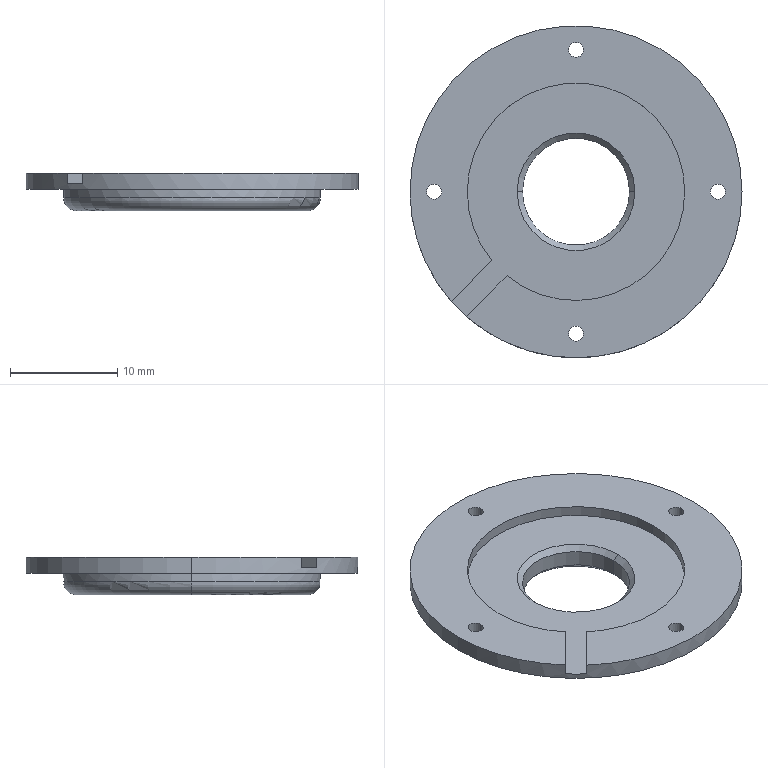Part | SolidWorks | features ICE 5, Chamfer 1, Extrusion 1, Fillet 1 | 1 solid | 41 faces | box 31 x 31 x 3.5 mm | volume 1459 mm3 | cylinder 25 | plane 10 | cone 4 | torus 2 | commonest cylinder face diameters 1.4 x8 2.5 x8 20.3 x3 10 x2 24 x2 31 x2
STEP:
#1=CARTESIAN_POINT('',(-5.,0.,2.));
#2=VERTEX_POINT('',#1);
#3=CARTESIAN_POINT('',(5.,0.,2.));
#4=VERTEX_POINT('',#3);
#5=CARTESIAN_POINT('',(0.,0.,2.));
#6=DIRECTION('',(0.,0.,1.));
#7=DIRECTION('',(1.,0.,0.));
#8=AXIS2_PLACEMENT_3D('',#5,#6,#7);
#9=CIRCLE('',#8,5.);
#10=EDGE_CURVE('',#2,#4,#9,.T.);
#11=ORIENTED_EDGE('',*,*,#10,.F.);
#12=CARTESIAN_POINT('',(-5.5,0.,2.5));
#13=VERTEX_POINT('',#12);
#14=CARTESIAN_POINT('',(-5.,0.,2.));
#15=DIRECTION('',(-0.7071,0.,0.7071));
#16=VECTOR('',#15,1000.);
#17=LINE('',#14,#16);
#18=EDGE_CURVE('',#2,#13,#17,.T.);
#19=ORIENTED_EDGE('',*,*,#18,.T.);
#20=CARTESIAN_POINT('',(5.5,0.,2.5));
#21=VERTEX_POINT('',#20);
#22=CARTESIAN_POINT('',(0.,0.,2.5));
#23=DIRECTION('',(0.,0.,-1.));
#24=DIRECTION('',(1.,0.,0.));
#25=AXIS2_PLACEMENT_3D('',#22,#23,#24);
#26=CIRCLE('',#25,5.5);
#27=EDGE_CURVE('',#21,#13,#26,.T.);
#28=ORIENTED_EDGE('',*,*,#27,.F.);
#29=CARTESIAN_POINT('',(5.,0.,2.));
#30=DIRECTION('',(0.7071,0.,0.7071));
#31=VECTOR('',#30,1000.);
#32=LINE('',#29,#31);
#33=EDGE_CURVE('',#4,#21,#32,.T.);
#34=ORIENTED_EDGE('',*,*,#33,.F.);
#35=EDGE_LOOP('',(#11,#19,#28,#34));
#36=FACE_OUTER_BOUND('',#35,.T.);
#37=CARTESIAN_POINT('',(0.,0.,2.));
#38=DIRECTION('',(0.,0.,1.));
#39=DIRECTION('',(1.,0.,0.));
#40=AXIS2_PLACEMENT_3D('',#37,#38,#39);
#41=CONICAL_SURFACE('',#40,5.,0.7854);
#42=ADVANCED_FACE('',(#36),#41,.F.);
#43=CARTESIAN_POINT('',(5.,0.,0.5));
#44=VERTEX_POINT('',#43);
#45=CARTESIAN_POINT('',(-5.,0.,0.5));
#46=VERTEX_POINT('',#45);
#47=CARTESIAN_POINT('',(0.,0.,0.5));
#48=DIRECTION('',(0.,0.,-1.));
#49=DIRECTION('',(1.,0.,0.));
#50=AXIS2_PLACEMENT_3D('',#47,#48,#49);
#51=CIRCLE('',#50,5.);
#52=EDGE_CURVE('',#44,#46,#51,.T.);
#53=ORIENTED_EDGE('',*,*,#52,.F.);
#54=CARTESIAN_POINT('',(5.5,0.,0.));
#55=VERTEX_POINT('',#54);
#56=CARTESIAN_POINT('',(5.,0.,0.5));
#57=DIRECTION('',(0.7071,0.,-0.7071));
#58=VECTOR('',#57,1000.);
#59=LINE('',#56,#58);
#60=EDGE_CURVE('',#44,#55,#59,.T.);
#61=ORIENTED_EDGE('',*,*,#60,.T.);
#62=CARTESIAN_POINT('',(-5.5,0.,0.));
#63=VERTEX_POINT('',#62);
#64=CARTESIAN_POINT('',(0.,0.,0.));
#65=DIRECTION('',(0.,0.,1.));
#66=DIRECTION('',(1.,0.,0.));
#67=AXIS2_PLACEMENT_3D('',#64,#65,#66);
#68=CIRCLE('',#67,5.5);
#69=EDGE_CURVE('',#63,#55,#68,.T.);
#70=ORIENTED_EDGE('',*,*,#69,.F.);
#71=CARTESIAN_POINT('',(-5.,0.,0.5));
#72=DIRECTION('',(-0.7071,0.,-0.7071));
#73=VECTOR('',#72,1000.);
#74=LINE('',#71,#73);
#75=EDGE_CURVE('',#46,#63,#74,.T.);
#76=ORIENTED_EDGE('',*,*,#75,.F.);
#77=EDGE_LOOP('',(#53,#61,#70,#76));
#78=FACE_OUTER_BOUND('',#77,.T.);
#79=CARTESIAN_POINT('',(0.,0.,0.5));
#80=DIRECTION('',(0.,0.,-1.));
#81=DIRECTION('',(-1.,0.,0.));
#82=AXIS2_PLACEMENT_3D('',#79,#80,#81);
#83=CONICAL_SURFACE('',#82,5.,0.7854);
#84=ADVANCED_FACE('',(#78),#83,.F.);
#85=ORIENTED_EDGE('',*,*,#10,.T.);
#86=CARTESIAN_POINT('',(5.,0.,3.5));
#87=DIRECTION('',(0.,0.,-1.));
#88=VECTOR('',#87,1000.);
#89=LINE('',#86,#88);
#90=EDGE_CURVE('',#4,#44,#89,.T.);
#91=ORIENTED_EDGE('',*,*,#90,.T.);
#92=ORIENTED_EDGE('',*,*,#52,.T.);
#93=CARTESIAN_POINT('',(-5.,0.,3.5));
#94=DIRECTION('',(0.,0.,-1.));
#95=VECTOR('',#94,1000.);
#96=LINE('',#93,#95);
#97=EDGE_CURVE('',#2,#46,#96,.T.);
#98=ORIENTED_EDGE('',*,*,#97,.F.);
#99=EDGE_LOOP('',(#85,#91,#92,#98));
#100=FACE_OUTER_BOUND('',#99,.T.);
#101=CARTESIAN_POINT('',(0.,0.,3.5));
#102=DIRECTION('',(0.,0.,-1.));
#103=DIRECTION('',(-1.,0.,0.));
#104=AXIS2_PLACEMENT_3D('',#101,#102,#103);
#105=CYLINDRICAL_SURFACE('',#104,5.);
#106=ADVANCED_FACE('',(#100),#105,.F.);
#107=CARTESIAN_POINT('',(1.25,13.25,2.5));
#108=VERTEX_POINT('',#107);
#109=CARTESIAN_POINT('',(-1.25,13.25,2.5));
#110=VERTEX_POINT('',#109);
#111=CARTESIAN_POINT('',(0.,13.25,2.5));
#112=DIRECTION('',(0.,0.,-1.));
#113=DIRECTION('',(-1.,0.,0.));
#114=AXIS2_PLACEMENT_3D('',#111,#112,#113);
#115=CIRCLE('',#114,1.25);
#116=EDGE_CURVE('',#108,#110,#115,.T.);
#117=ORIENTED_EDGE('',*,*,#116,.F.);
#118=CARTESIAN_POINT('',(1.25,13.25,2.));
#119=VERTEX_POINT('',#118);
#120=CARTESIAN_POINT('',(1.25,13.25,2.5));
#121=DIRECTION('',(0.,0.,-1.));
#122=VECTOR('',#121,1000.);
#123=LINE('',#120,#122);
#124=EDGE_CURVE('',#108,#119,#123,.T.);
#125=ORIENTED_EDGE('',*,*,#124,.T.);
#126=CARTESIAN_POINT('',(0.,12.,2.));
#127=VERTEX_POINT('',#126);
#128=CARTESIAN_POINT('',(0.,13.25,2.));
#129=DIRECTION('',(0.,0.,-1.));
#130=DIRECTION('',(-1.,0.,0.));
#131=AXIS2_PLACEMENT_3D('',#128,#129,#130);
#132=CIRCLE('',#131,1.25);
#133=EDGE_CURVE('',#119,#127,#132,.T.);
#134=ORIENTED_EDGE('',*,*,#133,.T.);
#135=CARTESIAN_POINT('',(-1.25,13.25,2.));
#136=VERTEX_POINT('',#135);
#137=CARTESIAN_POINT('',(0.,13.25,2.));
#138=DIRECTION('',(0.,0.,-1.));
#139=DIRECTION('',(-1.,0.,0.));
#140=AXIS2_PLACEMENT_3D('',#137,#138,#139);
#141=CIRCLE('',#140,1.25);
#142=EDGE_CURVE('',#127,#136,#141,.T.);
#143=ORIENTED_EDGE('',*,*,#142,.T.);
#144=CARTESIAN_POINT('',(-1.25,13.25,2.5));
#145=DIRECTION('',(0.,0.,-1.));
#146=VECTOR('',#145,1000.);
#147=LINE('',#144,#146);
#148=EDGE_CURVE('',#110,#136,#147,.T.);
#149=ORIENTED_EDGE('',*,*,#148,.F.);
#150=EDGE_LOOP('',(#117,#125,#134,#143,#149));
#151=FACE_OUTER_BOUND('',#150,.T.);
#152=CARTESIAN_POINT('',(0.,13.25,2.5));
#153=DIRECTION('',(0.,0.,-1.));
#154=DIRECTION('',(-1.,0.,0.));
#155=AXIS2_PLACEMENT_3D('',#152,#153,#154);
#156=CYLINDRICAL_SURFACE('',#155,1.25);
#157=ADVANCED_FACE('',(#151),#156,.F.);
#158=CARTESIAN_POINT('',(14.5,0.,2.5));
#159=VERTEX_POINT('',#158);
#160=CARTESIAN_POINT('',(12.,0.,2.5));
#161=VERTEX_POINT('',#160);
#162=CARTESIAN_POINT('',(13.25,0.,2.5));
#163=DIRECTION('',(0.,0.,-1.));
#164=DIRECTION('',(-1.,0.,0.));
#165=AXIS2_PLACEMENT_3D('',#162,#163,#164);
#166=CIRCLE('',#165,1.25);
#167=EDGE_CURVE('',#159,#161,#166,.T.);
#168=ORIENTED_EDGE('',*,*,#167,.F.);
#169=CARTESIAN_POINT('',(14.5,0.,2.));
#170=VERTEX_POINT('',#169);
#171=CARTESIAN_POINT('',(14.5,0.,2.5));
#172=DIRECTION('',(0.,0.,-1.));
#173=VECTOR('',#172,1000.);
#174=LINE('',#171,#173);
#175=EDGE_CURVE('',#159,#170,#174,.T.);
#176=ORIENTED_EDGE('',*,*,#175,.T.);
#177=CARTESIAN_POINT('',(12.,0.,2.));
#178=VERTEX_POINT('',#177);
#179=CARTESIAN_POINT('',(13.25,0.,2.));
#180=DIRECTION('',(0.,0.,-1.));
#181=DIRECTION('',(-1.,0.,0.));
#182=AXIS2_PLACEMENT_3D('',#179,#180,#181);
#183=CIRCLE('',#182,1.25);
#184=EDGE_CURVE('',#170,#178,#183,.T.);
#185=ORIENTED_EDGE('',*,*,#184,.T.);
#186=CARTESIAN_POINT('',(12.,0.,2.5));
#187=DIRECTION('',(0.,0.,-1.));
#188=VECTOR('',#187,1000.);
#189=LINE('',#186,#188);
#190=EDGE_CURVE('',#161,#178,#189,.T.);
#191=ORIENTED_EDGE('',*,*,#190,.F.);
#192=EDGE_LOOP('',(#168,#176,#185,#191));
#193=FACE_OUTER_BOUND('',#192,.T.);
#194=CARTESIAN_POINT('',(13.25,0.,2.5));
#195=DIRECTION('',(0.,0.,-1.));
#196=DIRECTION('',(-1.,0.,0.));
#197=AXIS2_PLACEMENT_3D('',#194,#195,#196);
#198=CYLINDRICAL_SURFACE('',#197,1.25);
#199=ADVANCED_FACE('',(#193),#198,.F.);
#200=CARTESIAN_POINT('',(1.25,-13.25,2.5));
#201=VERTEX_POINT('',#200);
#202=CARTESIAN_POINT('',(-1.25,-13.25,2.5));
#203=VERTEX_POINT('',#202);
#204=CARTESIAN_POINT('',(0.,-13.25,2.5));
#205=DIRECTION('',(0.,0.,-1.));
#206=DIRECTION('',(-1.,0.,0.));
#207=AXIS2_PLACEMENT_3D('',#204,#205,#206);
#208=CIRCLE('',#207,1.25);
#209=EDGE_CURVE('',#201,#203,#208,.T.);
#210=ORIENTED_EDGE('',*,*,#209,.F.);
#211=CARTESIAN_POINT('',(1.25,-13.25,2.));
#212=VERTEX_POINT('',#211);
#213=CARTESIAN_POINT('',(1.25,-13.25,2.5));
#214=DIRECTION('',(0.,0.,-1.));
#215=VECTOR('',#214,1000.);
#216=LINE('',#213,#215);
#217=EDGE_CURVE('',#201,#212,#216,.T.);
#218=ORIENTED_EDGE('',*,*,#217,.T.);
#219=CARTESIAN_POINT('',(-1.25,-13.25,2.));
#220=VERTEX_POINT('',#219);
#221=CARTESIAN_POINT('',(0.,-13.25,2.));
#222=DIRECTION('',(0.,0.,-1.));
#223=DIRECTION('',(-1.,0.,0.));
#224=AXIS2_PLACEMENT_3D('',#221,#222,#223);
#225=CIRCLE('',#224,1.25);
#226=EDGE_CURVE('',#212,#220,#225,.T.);
#227=ORIENTED_EDGE('',*,*,#226,.T.);
#228=CARTESIAN_POINT('',(-1.25,-13.25,2.5));
#229=DIRECTION('',(0.,0.,-1.));
#230=VECTOR('',#229,1000.);
#231=LINE('',#228,#230);
#232=EDGE_CURVE('',#203,#220,#231,.T.);
#233=ORIENTED_EDGE('',*,*,#232,.F.);
#234=EDGE_LOOP('',(#210,#218,#227,#233));
#235=FACE_OUTER_BOUND('',#234,.T.);
#236=CARTESIAN_POINT('',(0.,-13.25,2.5));
#237=DIRECTION('',(0.,0.,-1.));
#238=DIRECTION('',(-1.,0.,0.));
#239=AXIS2_PLACEMENT_3D('',#236,#237,#238);
#240=CYLINDRICAL_SURFACE('',#239,1.25);
#241=ADVANCED_FACE('',(#235),#240,.F.);
#242=CARTESIAN_POINT('',(-12.,0.,2.5));
#243=VERTEX_POINT('',#242);
#244=CARTESIAN_POINT('',(-14.5,0.,2.5));
#245=VERTEX_POINT('',#244);
#246=CARTESIAN_POINT('',(-13.25,0.,2.5));
#247=DIRECTION('',(0.,0.,-1.));
#248=DIRECTION('',(-1.,0.,0.));
#249=AXIS2_PLACEMENT_3D('',#246,#247,#248);
#250=CIRCLE('',#249,1.25);
#251=EDGE_CURVE('',#243,#245,#250,.T.);
#252=ORIENTED_EDGE('',*,*,#251,.F.);
#253=CARTESIAN_POINT('',(-12.,0.,2.));
#254=VERTEX_POINT('',#253);
#255=CARTESIAN_POINT('',(-12.,0.,2.5));
#256=DIRECTION('',(0.,0.,-1.));
#257=VECTOR('',#256,1000.);
#258=LINE('',#255,#257);
#259=EDGE_CURVE('',#243,#254,#258,.T.);
#260=ORIENTED_EDGE('',*,*,#259,.T.);
#261=CARTESIAN_POINT('',(-14.5,0.,2.));
#262=VERTEX_POINT('',#261);
#263=CARTESIAN_POINT('',(-13.25,0.,2.));
#264=DIRECTION('',(0.,0.,-1.));
#265=DIRECTION('',(-1.,0.,0.));
#266=AXIS2_PLACEMENT_3D('',#263,#264,#265);
#267=CIRCLE('',#266,1.25);
#268=EDGE_CURVE('',#254,#262,#267,.T.);
#269=ORIENTED_EDGE('',*,*,#268,.T.);
#270=CARTESIAN_POINT('',(-14.5,0.,2.5));
#271=DIRECTION('',(0.,0.,-1.));
#272=VECTOR('',#271,1000.);
#273=LINE('',#270,#272);
#274=EDGE_CURVE('',#245,#262,#273,.T.);
#275=ORIENTED_EDGE('',*,*,#274,.F.);
#276=EDGE_LOOP('',(#252,#260,#269,#275));
#277=FACE_OUTER_BOUND('',#276,.T.);
#278=CARTESIAN_POINT('',(-13.25,0.,2.5));
#279=DIRECTION('',(0.,0.,-1.));
#280=DIRECTION('',(-1.,0.,0.));
#281=AXIS2_PLACEMENT_3D('',#278,#279,#280);
#282=CYLINDRICAL_SURFACE('',#281,1.25);
#283=ADVANCED_FACE('',(#277),#282,.F.);
#284=CARTESIAN_POINT('',(-10.8,0.,0.));
#285=VERTEX_POINT('',#284);
#286=CARTESIAN_POINT('',(10.8,0.,0.));
#287=VERTEX_POINT('',#286);
#288=CARTESIAN_POINT('',(0.,0.,0.));
#289=DIRECTION('',(0.,0.,-1.));
#290=DIRECTION('',(1.,0.,0.));
#291=AXIS2_PLACEMENT_3D('',#288,#289,#290);
#292=CIRCLE('',#291,10.8);
#293=EDGE_CURVE('',#285,#287,#292,.T.);
#294=ORIENTED_EDGE('',*,*,#293,.F.);
#295=CARTESIAN_POINT('',(-12.,0.,1.2));
#296=VERTEX_POINT('',#295);
#297=CARTESIAN_POINT('',(-10.8,0.,1.2));
#298=DIRECTION('',(0.,1.,0.));
#299=DIRECTION('',(-1.,0.,0.));
#300=AXIS2_PLACEMENT_3D('',#297,#298,#299);
#301=CIRCLE('',#300,1.2);
#302=EDGE_CURVE('',#285,#296,#301,.T.);
#303=ORIENTED_EDGE('',*,*,#302,.T.);
#304=CARTESIAN_POINT('',(12.,0.,1.2));
#305=VERTEX_POINT('',#304);
#306=CARTESIAN_POINT('',(0.,0.,1.2));
#307=DIRECTION('',(0.,0.,1.));
#308=DIRECTION('',(1.,0.,0.));
#309=AXIS2_PLACEMENT_3D('',#306,#307,#308);
#310=CIRCLE('',#309,12.);
#311=EDGE_CURVE('',#305,#296,#310,.T.);
#312=ORIENTED_EDGE('',*,*,#311,.F.);
#313=CARTESIAN_POINT('',(10.8,0.,1.2));
#314=DIRECTION('',(0.,-1.,0.));
#315=DIRECTION('',(0.,0.,-1.));
#316=AXIS2_PLACEMENT_3D('',#313,#314,#315);
#317=CIRCLE('',#316,1.2);
#318=EDGE_CURVE('',#287,#305,#317,.T.);
#319=ORIENTED_EDGE('',*,*,#318,.F.);
#320=EDGE_LOOP('',(#294,#303,#312,#319));
#321=FACE_OUTER_BOUND('',#320,.T.);
#322=CARTESIAN_POINT('',(0.,0.,1.2));
#323=DIRECTION('',(0.,0.,1.));
#324=DIRECTION('',(1.,0.,0.));
#325=AXIS2_PLACEMENT_3D('',#322,#323,#324);
#326=TOROIDAL_SURFACE('',#325,10.8,1.2);
#327=ADVANCED_FACE('',(#321),#326,.T.);
#328=CARTESIAN_POINT('',(-10.15,0.,2.5));
#329=VERTEX_POINT('',#328);
#330=CARTESIAN_POINT('',(-7.849,-6.435,2.5));
#331=VERTEX_POINT('',#330);
#332=CARTESIAN_POINT('',(0.,0.,2.5));
#333=DIRECTION('',(0.,0.,1.));
#334=DIRECTION('',(1.,0.,0.));
#335=AXIS2_PLACEMENT_3D('',#332,#333,#334);
#336=CIRCLE('',#335,10.15);
#337=EDGE_CURVE('',#329,#331,#336,.T.);
#338=ORIENTED_EDGE('',*,*,#337,.F.);
#339=CARTESIAN_POINT('',(-10.15,0.,3.5));
#340=VERTEX_POINT('',#339);
#341=CARTESIAN_POINT('',(-10.15,0.,2.5));
#342=DIRECTION('',(0.,0.,1.));
#343=VECTOR('',#342,1000.);
#344=LINE('',#341,#343);
#345=EDGE_CURVE('',#329,#340,#344,.T.);
#346=ORIENTED_EDGE('',*,*,#345,.T.);
#347=CARTESIAN_POINT('',(-7.849,-6.435,3.5));
#348=VERTEX_POINT('',#347);
#349=CARTESIAN_POINT('',(0.,0.,3.5));
#350=DIRECTION('',(0.,0.,1.));
#351=DIRECTION('',(1.,0.,0.));
#352=AXIS2_PLACEMENT_3D('',#349,#350,#351);
#353=CIRCLE('',#352,10.15);
#354=EDGE_CURVE('',#340,#348,#353,.T.);
#355=ORIENTED_EDGE('',*,*,#354,.T.);
#356=CARTESIAN_POINT('',(-7.849,-6.435,2.5));
#357=DIRECTION('',(0.,0.,-1.));
#358=VECTOR('',#357,1000.);
#359=LINE('',#356,#358);
#360=EDGE_CURVE('',#348,#331,#359,.T.);
#361=ORIENTED_EDGE('',*,*,#360,.T.);
#362=EDGE_LOOP('',(#338,#346,#355,#361));
#363=FACE_OUTER_BOUND('',#362,.T.);
#364=CARTESIAN_POINT('',(0.,0.,2.5));
#365=DIRECTION('',(0.,0.,1.));
#366=DIRECTION('',(1.,0.,0.));
#367=AXIS2_PLACEMENT_3D('',#364,#365,#366);
#368=CYLINDRICAL_SURFACE('',#367,10.15);
#369=ADVANCED_FACE('',(#363),#368,.F.);
#370=ORIENTED_EDGE('',*,*,#345,.F.);
#371=CARTESIAN_POINT('',(10.15,0.,2.5));
#372=VERTEX_POINT('',#371);
#373=CARTESIAN_POINT('',(0.,0.,2.5));
#374=DIRECTION('',(0.,0.,1.));
#375=DIRECTION('',(1.,0.,0.));
#376=AXIS2_PLACEMENT_3D('',#373,#374,#375);
#377=CIRCLE('',#376,10.15);
#378=EDGE_CURVE('',#372,#329,#377,.T.);
#379=ORIENTED_EDGE('',*,*,#378,.F.);
#380=CARTESIAN_POINT('',(10.15,0.,3.5));
#381=VERTEX_POINT('',#380);
#382=CARTESIAN_POINT('',(10.15,0.,2.5));
#383=DIRECTION('',(0.,0.,1.));
#384=VECTOR('',#383,1000.);
#385=LINE('',#382,#384);
#386=EDGE_CURVE('',#372,#381,#385,.T.);
#387=ORIENTED_EDGE('',*,*,#386,.T.);
#388=CARTESIAN_POINT('',(0.,0.,3.5));
#389=DIRECTION('',(0.,0.,1.));
#390=DIRECTION('',(1.,0.,0.));
#391=AXIS2_PLACEMENT_3D('',#388,#389,#390);
#392=CIRCLE('',#391,10.15);
#393=EDGE_CURVE('',#381,#340,#392,.T.);
#394=ORIENTED_EDGE('',*,*,#393,.T.);
#395=EDGE_LOOP('',(#370,#379,#387,#394));
#396=FACE_OUTER_BOUND('',#395,.T.);
#397=CARTESIAN_POINT('',(0.,0.,2.5));
#398=DIRECTION('',(0.,0.,1.));
#399=DIRECTION('',(1.,0.,0.));
#400=AXIS2_PLACEMENT_3D('',#397,#398,#399);
#401=CYLINDRICAL_SURFACE('',#400,10.15);
#402=ADVANCED_FACE('',(#396),#401,.F.);
#403=CARTESIAN_POINT('',(15.5,0.,3.5));
#404=VERTEX_POINT('',#403);
#405=CARTESIAN_POINT('',(-15.5,0.,3.5));
#406=VERTEX_POINT('',#405);
#407=CARTESIAN_POINT('',(0.,0.,3.5));
#408=DIRECTION('',(0.,0.,1.));
#409=DIRECTION('',(1.,0.,0.));
#410=AXIS2_PLACEMENT_3D('',#407,#408,#409);
#411=CIRCLE('',#410,15.5);
#412=EDGE_CURVE('',#404,#406,#411,.T.);
#413=ORIENTED_EDGE('',*,*,#412,.F.);
#414=CARTESIAN_POINT('',(15.5,0.,2.));
#415=VERTEX_POINT('',#414);
#416=CARTESIAN_POINT('',(15.5,0.,3.5));
#417=DIRECTION('',(0.,0.,-1.));
#418=VECTOR('',#417,1000.);
#419=LINE('',#416,#418);
#420=EDGE_CURVE('',#404,#415,#419,.T.);
#421=ORIENTED_EDGE('',*,*,#420,.T.);
#422=CARTESIAN_POINT('',(-15.5,0.,2.));
#423=VERTEX_POINT('',#422);
#424=CARTESIAN_POINT('',(0.,0.,2.));
#425=DIRECTION('',(0.,0.,1.));
#426=DIRECTION('',(1.,0.,0.));
#427=AXIS2_PLACEMENT_3D('',#424,#425,#426);
#428=CIRCLE('',#427,15.5);
#429=EDGE_CURVE('',#415,#423,#428,.T.);
#430=ORIENTED_EDGE('',*,*,#429,.T.);
#431=CARTESIAN_POINT('',(-15.5,0.,3.5));
#432=DIRECTION('',(0.,0.,-1.));
#433=VECTOR('',#432,1000.);
#434=LINE('',#431,#433);
#435=EDGE_CURVE('',#406,#423,#434,.T.);
#436=ORIENTED_EDGE('',*,*,#435,.F.);
#437=EDGE_LOOP('',(#413,#421,#430,#436));
#438=FACE_OUTER_BOUND('',#437,.T.);
#439=CARTESIAN_POINT('',(0.,0.,3.5));
#440=DIRECTION('',(0.,0.,-1.));
#441=DIRECTION('',(-1.,0.,0.));
#442=AXIS2_PLACEMENT_3D('',#439,#440,#441);
#443=CYLINDRICAL_SURFACE('',#442,15.5);
#444=ADVANCED_FACE('',(#438),#443,.T.);
#445=CARTESIAN_POINT('',(0.,0.,2.));
#446=DIRECTION('',(0.,0.,1.));
#447=DIRECTION('',(1.,0.,0.));
#448=AXIS2_PLACEMENT_3D('',#445,#446,#447);
#449=CIRCLE('',#448,12.);
#450=EDGE_CURVE('',#178,#127,#449,.T.);
#451=ORIENTED_EDGE('',*,*,#450,.F.);
#452=CARTESIAN_POINT('',(12.,0.,2.));
#453=DIRECTION('',(0.,0.,-1.));
#454=VECTOR('',#453,1000.);
#455=LINE('',#452,#454);
#456=EDGE_CURVE('',#178,#305,#455,.T.);
#457=ORIENTED_EDGE('',*,*,#456,.T.);
#458=ORIENTED_EDGE('',*,*,#311,.T.);
#459=CARTESIAN_POINT('',(-12.,0.,2.));
#460=DIRECTION('',(0.,0.,-1.));
#461=VECTOR('',#460,1000.);
#462=LINE('',#459,#461);
#463=EDGE_CURVE('',#254,#296,#462,.T.);
#464=ORIENTED_EDGE('',*,*,#463,.F.);
#465=CARTESIAN_POINT('',(0.,0.,2.));
#466=DIRECTION('',(0.,0.,1.));
#467=DIRECTION('',(1.,0.,0.));
#468=AXIS2_PLACEMENT_3D('',#465,#466,#467);
#469=CIRCLE('',#468,12.);
#470=EDGE_CURVE('',#127,#254,#469,.T.);
#471=ORIENTED_EDGE('',*,*,#470,.F.);
#472=EDGE_LOOP('',(#451,#457,#458,#464,#471));
#473=FACE_OUTER_BOUND('',#472,.T.);
#474=CARTESIAN_POINT('',(0.,0.,2.));
#475=DIRECTION('',(0.,0.,-1.));
#476=DIRECTION('',(-1.,0.,0.));
#477=AXIS2_PLACEMENT_3D('',#474,#475,#476);
#478=CYLINDRICAL_SURFACE('',#477,12.);
#479=ADVANCED_FACE('',(#473),#478,.T.);
#480=CARTESIAN_POINT('',(-13.95,0.,3.5));
#481=VERTEX_POINT('',#480);
#482=CARTESIAN_POINT('',(-12.55,0.,3.5));
#483=VERTEX_POINT('',#482);
#484=CARTESIAN_POINT('',(-13.25,0.,3.5));
#485=DIRECTION('',(0.,0.,1.));
#486=DIRECTION('',(1.,0.,0.));
#487=AXIS2_PLACEMENT_3D('',#484,#485,#486);
#488=CIRCLE('',#487,0.7);
#489=EDGE_CURVE('',#481,#483,#488,.T.);
#490=ORIENTED_EDGE('',*,*,#489,.T.);
#491=CARTESIAN_POINT('',(-12.55,0.,2.5));
#492=VERTEX_POINT('',#491);
#493=CARTESIAN_POINT('',(-12.55,0.,3.5));
#494=DIRECTION('',(0.,0.,-1.));
#495=VECTOR('',#494,1000.);
#496=LINE('',#493,#495);
#497=EDGE_CURVE('',#483,#492,#496,.T.);
#498=ORIENTED_EDGE('',*,*,#497,.T.);
#499=CARTESIAN_POINT('',(-13.95,0.,2.5));
#500=VERTEX_POINT('',#499);
#501=CARTESIAN_POINT('',(-13.25,0.,2.5));
#502=DIRECTION('',(0.,0.,-1.));
#503=DIRECTION('',(-1.,0.,0.));
#504=AXIS2_PLACEMENT_3D('',#501,#502,#503);
#505=CIRCLE('',#504,0.7);
#506=EDGE_CURVE('',#492,#500,#505,.T.);
#507=ORIENTED_EDGE('',*,*,#506,.T.);
#508=CARTESIAN_POINT('',(-13.95,0.,3.5));
#509=DIRECTION('',(0.,0.,-1.));
#510=VECTOR('',#509,1000.);
#511=LINE('',#508,#510);
#512=EDGE_CURVE('',#481,#500,#511,.T.);
#513=ORIENTED_EDGE('',*,*,#512,.F.);
#514=EDGE_LOOP('',(#490,#498,#507,#513));
#515=FACE_OUTER_BOUND('',#514,.T.);
#516=CARTESIAN_POINT('',(-13.25,0.,3.5));
#517=DIRECTION('',(0.,0.,-1.));
#518=DIRECTION('',(-1.,0.,0.));
#519=AXIS2_PLACEMENT_3D('',#516,#517,#518);
#520=CYLINDRICAL_SURFACE('',#519,0.7);
#521=ADVANCED_FACE('',(#515),#520,.F.);
#522=CARTESIAN_POINT('',(-0.7,-13.25,3.5));
#523=VERTEX_POINT('',#522);
#524=CARTESIAN_POINT('',(0.7,-13.25,3.5));
#525=VERTEX_POINT('',#524);
#526=CARTESIAN_POINT('',(0.,-13.25,3.5));
#527=DIRECTION('',(0.,0.,1.));
#528=DIRECTION('',(1.,0.,0.));
#529=AXIS2_PLACEMENT_3D('',#526,#527,#528);
#530=CIRCLE('',#529,0.7);
#531=EDGE_CURVE('',#523,#525,#530,.T.);
#532=ORIENTED_EDGE('',*,*,#531,.T.);
#533=CARTESIAN_POINT('',(0.7,-13.25,2.5));
#534=VERTEX_POINT('',#533);
#535=CARTESIAN_POINT('',(0.7,-13.25,3.5));
#536=DIRECTION('',(0.,0.,-1.));
#537=VECTOR('',#536,1000.);
#538=LINE('',#535,#537);
#539=EDGE_CURVE('',#525,#534,#538,.T.);
#540=ORIENTED_EDGE('',*,*,#539,.T.);
#541=CARTESIAN_POINT('',(-0.7,-13.25,2.5));
#542=VERTEX_POINT('',#541);
#543=CARTESIAN_POINT('',(0.,-13.25,2.5));
#544=DIRECTION('',(0.,0.,-1.));
#545=DIRECTION('',(-1.,0.,0.));
#546=AXIS2_PLACEMENT_3D('',#543,#544,#545);
#547=CIRCLE('',#546,0.7);
#548=EDGE_CURVE('',#534,#542,#547,.T.);
#549=ORIENTED_EDGE('',*,*,#548,.T.);
#550=CARTESIAN_POINT('',(-0.7,-13.25,3.5));
#551=DIRECTION('',(0.,0.,-1.));
#552=VECTOR('',#551,1000.);
#553=LINE('',#550,#552);
#554=EDGE_CURVE('',#523,#542,#553,.T.);
#555=ORIENTED_EDGE('',*,*,#554,.F.);
#556=EDGE_LOOP('',(#532,#540,#549,#555));
#557=FACE_OUTER_BOUND('',#556,.T.);
#558=CARTESIAN_POINT('',(0.,-13.25,3.5));
#559=DIRECTION('',(0.,0.,-1.));
#560=DIRECTION('',(-1.,0.,0.));
#561=AXIS2_PLACEMENT_3D('',#558,#559,#560);
#562=CYLINDRICAL_SURFACE('',#561,0.7);
#563=ADVANCED_FACE('',(#557),#562,.F.);
#564=CARTESIAN_POINT('',(12.55,0.,3.5));
#565=VERTEX_POINT('',#564);
#566=CARTESIAN_POINT('',(13.95,0.,3.5));
#567=VERTEX_POINT('',#566);
#568=CARTESIAN_POINT('',(13.25,0.,3.5));
#569=DIRECTION('',(0.,0.,1.));
#570=DIRECTION('',(1.,0.,0.));
#571=AXIS2_PLACEMENT_3D('',#568,#569,#570);
#572=CIRCLE('',#571,0.7);
#573=EDGE_CURVE('',#565,#567,#572,.T.);
#574=ORIENTED_EDGE('',*,*,#573,.T.);
#575=CARTESIAN_POINT('',(13.95,0.,2.5));
#576=VERTEX_POINT('',#575);
#577=CARTESIAN_POINT('',(13.95,0.,3.5));
#578=DIRECTION('',(0.,0.,-1.));
#579=VECTOR('',#578,1000.);
#580=LINE('',#577,#579);
#581=EDGE_CURVE('',#567,#576,#580,.T.);
#582=ORIENTED_EDGE('',*,*,#581,.T.);
#583=CARTESIAN_POINT('',(12.55,0.,2.5));
#584=VERTEX_POINT('',#583);
#585=CARTESIAN_POINT('',(13.25,0.,2.5));
#586=DIRECTION('',(0.,0.,-1.));
#587=DIRECTION('',(-1.,0.,0.));
#588=AXIS2_PLACEMENT_3D('',#585,#586,#587);
#589=CIRCLE('',#588,0.7);
#590=EDGE_CURVE('',#576,#584,#589,.T.);
#591=ORIENTED_EDGE('',*,*,#590,.T.);
#592=CARTESIAN_POINT('',(12.55,0.,3.5));
#593=DIRECTION('',(0.,0.,-1.));
#594=VECTOR('',#593,1000.);
#595=LINE('',#592,#594);
#596=EDGE_CURVE('',#565,#584,#595,.T.);
#597=ORIENTED_EDGE('',*,*,#596,.F.);
#598=EDGE_LOOP('',(#574,#582,#591,#597));
#599=FACE_OUTER_BOUND('',#598,.T.);
#600=CARTESIAN_POINT('',(13.25,0.,3.5));
#601=DIRECTION('',(0.,0.,-1.));
#602=DIRECTION('',(-1.,0.,0.));
#603=AXIS2_PLACEMENT_3D('',#600,#601,#602);
#604=CYLINDRICAL_SURFACE('',#603,0.7);
#605=ADVANCED_FACE('',(#599),#604,.F.);
#606=CARTESIAN_POINT('',(-0.7,13.25,3.5));
#607=VERTEX_POINT('',#606);
#608=CARTESIAN_POINT('',(0.7,13.25,3.5));
#609=VERTEX_POINT('',#608);
#610=CARTESIAN_POINT('',(0.,13.25,3.5));
#611=DIRECTION('',(0.,0.,1.));
#612=DIRECTION('',(1.,0.,0.));
#613=AXIS2_PLACEMENT_3D('',#610,#611,#612);
#614=CIRCLE('',#613,0.7);
#615=EDGE_CURVE('',#607,#609,#614,.T.);
#616=ORIENTED_EDGE('',*,*,#615,.T.);
#617=CARTESIAN_POINT('',(0.7,13.25,2.5));
#618=VERTEX_POINT('',#617);
#619=CARTESIAN_POINT('',(0.7,13.25,3.5));
#620=DIRECTION('',(0.,0.,-1.));
#621=VECTOR('',#620,1000.);
#622=LINE('',#619,#621);
#623=EDGE_CURVE('',#609,#618,#622,.T.);
#624=ORIENTED_EDGE('',*,*,#623,.T.);
#625=CARTESIAN_POINT('',(-0.7,13.25,2.5));
#626=VERTEX_POINT('',#625);
#627=CARTESIAN_POINT('',(0.,13.25,2.5));
#628=DIRECTION('',(0.,0.,-1.));
#629=DIRECTION('',(-1.,0.,0.));
#630=AXIS2_PLACEMENT_3D('',#627,#628,#629);
#631=CIRCLE('',#630,0.7);
#632=EDGE_CURVE('',#618,#626,#631,.T.);
#633=ORIENTED_EDGE('',*,*,#632,.T.);
#634=CARTESIAN_POINT('',(-0.7,13.25,3.5));
#635=DIRECTION('',(0.,0.,-1.));
#636=VECTOR('',#635,1000.);
#637=LINE('',#634,#636);
#638=EDGE_CURVE('',#607,#626,#637,.T.);
#639=ORIENTED_EDGE('',*,*,#638,.F.);
#640=EDGE_LOOP('',(#616,#624,#633,#639));
#641=FACE_OUTER_BOUND('',#640,.T.);
#642=CARTESIAN_POINT('',(0.,13.25,3.5));
#643=DIRECTION('',(0.,0.,-1.));
#644=DIRECTION('',(-1.,0.,0.));
#645=AXIS2_PLACEMENT_3D('',#642,#643,#644);
#646=CYLINDRICAL_SURFACE('',#645,0.7);
#647=ADVANCED_FACE('',(#641),#646,.F.);
#648=ORIENTED_EDGE('',*,*,#623,.F.);
#649=CARTESIAN_POINT('',(0.,13.25,3.5));
#650=DIRECTION('',(0.,0.,1.));
#651=DIRECTION('',(1.,0.,0.));
#652=AXIS2_PLACEMENT_3D('',#649,#650,#651);
#653=CIRCLE('',#652,0.7);
#654=EDGE_CURVE('',#609,#607,#653,.T.);
#655=ORIENTED_EDGE('',*,*,#654,.T.);
#656=ORIENTED_EDGE('',*,*,#638,.T.);
#657=CARTESIAN_POINT('',(0.,13.25,2.5));
#658=DIRECTION('',(0.,0.,-1.));
#659=DIRECTION('',(-1.,0.,0.));
#660=AXIS2_PLACEMENT_3D('',#657,#658,#659);
#661=CIRCLE('',#660,0.7);
#662=EDGE_CURVE('',#626,#618,#661,.T.);
#663=ORIENTED_EDGE('',*,*,#662,.T.);
#664=EDGE_LOOP('',(#648,#655,#656,#663));
#665=FACE_OUTER_BOUND('',#664,.T.);
#666=CARTESIAN_POINT('',(0.,13.25,3.5));
#667=DIRECTION('',(0.,0.,-1.));
#668=DIRECTION('',(-1.,0.,0.));
#669=AXIS2_PLACEMENT_3D('',#666,#667,#668);
#670=CYLINDRICAL_SURFACE('',#669,0.7);
#671=ADVANCED_FACE('',(#665),#670,.F.);
#672=ORIENTED_EDGE('',*,*,#581,.F.);
#673=CARTESIAN_POINT('',(13.25,0.,3.5));
#674=DIRECTION('',(0.,0.,1.));
#675=DIRECTION('',(1.,0.,0.));
#676=AXIS2_PLACEMENT_3D('',#673,#674,#675);
#677=CIRCLE('',#676,0.7);
#678=EDGE_CURVE('',#567,#565,#677,.T.);
#679=ORIENTED_EDGE('',*,*,#678,.T.);
#680=ORIENTED_EDGE('',*,*,#596,.T.);
#681=CARTESIAN_POINT('',(13.25,0.,2.5));
#682=DIRECTION('',(0.,0.,-1.));
#683=DIRECTION('',(-1.,0.,0.));
#684=AXIS2_PLACEMENT_3D('',#681,#682,#683);
#685=CIRCLE('',#684,0.7);
#686=EDGE_CURVE('',#584,#576,#685,.T.);
#687=ORIENTED_EDGE('',*,*,#686,.T.);
#688=EDGE_LOOP('',(#672,#679,#680,#687));
#689=FACE_OUTER_BOUND('',#688,.T.);
#690=CARTESIAN_POINT('',(13.25,0.,3.5));
#691=DIRECTION('',(0.,0.,-1.));
#692=DIRECTION('',(-1.,0.,0.));
#693=AXIS2_PLACEMENT_3D('',#690,#691,#692);
#694=CYLINDRICAL_SURFACE('',#693,0.7);
#695=ADVANCED_FACE('',(#689),#694,.F.);
#696=ORIENTED_EDGE('',*,*,#539,.F.);
#697=CARTESIAN_POINT('',(0.,-13.25,3.5));
#698=DIRECTION('',(0.,0.,1.));
#699=DIRECTION('',(1.,0.,0.));
#700=AXIS2_PLACEMENT_3D('',#697,#698,#699);
#701=CIRCLE('',#700,0.7);
#702=EDGE_CURVE('',#525,#523,#701,.T.);
#703=ORIENTED_EDGE('',*,*,#702,.T.);
#704=ORIENTED_EDGE('',*,*,#554,.T.);
#705=CARTESIAN_POINT('',(0.,-13.25,2.5));
#706=DIRECTION('',(0.,0.,-1.));
#707=DIRECTION('',(-1.,0.,0.));
#708=AXIS2_PLACEMENT_3D('',#705,#706,#707);
#709=CIRCLE('',#708,0.7);
#710=EDGE_CURVE('',#542,#534,#709,.T.);
#711=ORIENTED_EDGE('',*,*,#710,.T.);
#712=EDGE_LOOP('',(#696,#703,#704,#711));
#713=FACE_OUTER_BOUND('',#712,.T.);
#714=CARTESIAN_POINT('',(0.,-13.25,3.5));
#715=DIRECTION('',(0.,0.,-1.));
#716=DIRECTION('',(-1.,0.,0.));
#717=AXIS2_PLACEMENT_3D('',#714,#715,#716);
#718=CYLINDRICAL_SURFACE('',#717,0.7);
#719=ADVANCED_FACE('',(#713),#718,.F.);
#720=ORIENTED_EDGE('',*,*,#497,.F.);
#721=CARTESIAN_POINT('',(-13.25,0.,3.5));
#722=DIRECTION('',(0.,0.,1.));
#723=DIRECTION('',(1.,0.,0.));
#724=AXIS2_PLACEMENT_3D('',#721,#722,#723);
#725=CIRCLE('',#724,0.7);
#726=EDGE_CURVE('',#483,#481,#725,.T.);
#727=ORIENTED_EDGE('',*,*,#726,.T.);
#728=ORIENTED_EDGE('',*,*,#512,.T.);
#729=CARTESIAN_POINT('',(-13.25,0.,2.5));
#730=DIRECTION('',(0.,0.,-1.));
#731=DIRECTION('',(-1.,0.,0.));
#732=AXIS2_PLACEMENT_3D('',#729,#730,#731);
#733=CIRCLE('',#732,0.7);
#734=EDGE_CURVE('',#500,#492,#733,.T.);
#735=ORIENTED_EDGE('',*,*,#734,.T.);
#736=EDGE_LOOP('',(#720,#727,#728,#735));
#737=FACE_OUTER_BOUND('',#736,.T.);
#738=CARTESIAN_POINT('',(-13.25,0.,3.5));
#739=DIRECTION('',(0.,0.,-1.));
#740=DIRECTION('',(-1.,0.,0.));
#741=AXIS2_PLACEMENT_3D('',#738,#739,#740);
#742=CYLINDRICAL_SURFACE('',#741,0.7);
#743=ADVANCED_FACE('',(#737),#742,.F.);
#744=ORIENTED_EDGE('',*,*,#456,.F.);
#745=CARTESIAN_POINT('',(0.,-12.,2.));
#746=VERTEX_POINT('',#745);
#747=CARTESIAN_POINT('',(0.,0.,2.));
#748=DIRECTION('',(0.,0.,1.));
#749=DIRECTION('',(1.,0.,0.));
#750=AXIS2_PLACEMENT_3D('',#747,#748,#749);
#751=CIRCLE('',#750,12.);
#752=EDGE_CURVE('',#746,#178,#751,.T.);
#753=ORIENTED_EDGE('',*,*,#752,.F.);
#754=CARTESIAN_POINT('',(0.,0.,2.));
#755=DIRECTION('',(0.,0.,1.));
#756=DIRECTION('',(1.,0.,0.));
#757=AXIS2_PLACEMENT_3D('',#754,#755,#756);
#758=CIRCLE('',#757,12.);
#759=EDGE_CURVE('',#254,#746,#758,.T.);
#760=ORIENTED_EDGE('',*,*,#759,.F.);
#761=ORIENTED_EDGE('',*,*,#463,.T.);
#762=CARTESIAN_POINT('',(0.,0.,1.2));
#763=DIRECTION('',(0.,0.,1.));
#764=DIRECTION('',(1.,0.,0.));
#765=AXIS2_PLACEMENT_3D('',#762,#763,#764);
#766=CIRCLE('',#765,12.);
#767=EDGE_CURVE('',#296,#305,#766,.T.);
#768=ORIENTED_EDGE('',*,*,#767,.T.);
#769=EDGE_LOOP('',(#744,#753,#760,#761,#768));
#770=FACE_OUTER_BOUND('',#769,.T.);
#771=CARTESIAN_POINT('',(0.,0.,2.));
#772=DIRECTION('',(0.,0.,-1.));
#773=DIRECTION('',(-1.,0.,0.));
#774=AXIS2_PLACEMENT_3D('',#771,#772,#773);
#775=CYLINDRICAL_SURFACE('',#774,12.);
#776=ADVANCED_FACE('',(#770),#775,.T.);
#777=ORIENTED_EDGE('',*,*,#69,.T.);
#778=CARTESIAN_POINT('',(0.,0.,0.));
#779=DIRECTION('',(0.,0.,1.));
#780=DIRECTION('',(1.,0.,0.));
#781=AXIS2_PLACEMENT_3D('',#778,#779,#780);
#782=CIRCLE('',#781,5.5);
#783=EDGE_CURVE('',#55,#63,#782,.T.);
#784=ORIENTED_EDGE('',*,*,#783,.T.);
#785=EDGE_LOOP('',(#777,#784));
#786=FACE_BOUND('',#785,.T.);
#787=CARTESIAN_POINT('',(0.,0.,0.));
#788=DIRECTION('',(0.,0.,-1.));
#789=DIRECTION('',(1.,0.,0.));
#790=AXIS2_PLACEMENT_3D('',#787,#788,#789);
#791=CIRCLE('',#790,10.8);
#792=EDGE_CURVE('',#287,#285,#791,.T.);
#793=ORIENTED_EDGE('',*,*,#792,.T.);
#794=ORIENTED_EDGE('',*,*,#293,.T.);
#795=EDGE_LOOP('',(#793,#794));
#796=FACE_OUTER_BOUND('',#795,.T.);
#797=CARTESIAN_POINT('',(0.,0.,0.));
#798=DIRECTION('',(0.,0.,1.));
#799=DIRECTION('',(1.,0.,0.));
#800=AXIS2_PLACEMENT_3D('',#797,#798,#799);
#801=PLANE('',#800);
#802=ADVANCED_FACE('',(#786,#796),#801,.F.);
#803=CARTESIAN_POINT('',(-11.644,-10.23,3.5));
#804=VERTEX_POINT('',#803);
#805=CARTESIAN_POINT('',(-0.7071,0.7071,3.5));
#806=DIRECTION('',(-0.7071,-0.7071,0.));
#807=VECTOR('',#806,1000.);
#808=LINE('',#805,#807);
#809=EDGE_CURVE('',#348,#804,#808,.T.);
#810=ORIENTED_EDGE('',*,*,#809,.F.);
#811=ORIENTED_EDGE('',*,*,#354,.F.);
#812=ORIENTED_EDGE('',*,*,#393,.F.);
#813=CARTESIAN_POINT('',(-6.435,-7.849,3.5));
#814=VERTEX_POINT('',#813);
#815=CARTESIAN_POINT('',(0.,0.,3.5));
#816=DIRECTION('',(0.,0.,1.));
#817=DIRECTION('',(1.,0.,0.));
#818=AXIS2_PLACEMENT_3D('',#815,#816,#817);
#819=CIRCLE('',#818,10.15);
#820=EDGE_CURVE('',#814,#381,#819,.T.);
#821=ORIENTED_EDGE('',*,*,#820,.F.);
#822=CARTESIAN_POINT('',(-10.23,-11.644,3.5));
#823=VERTEX_POINT('',#822);
#824=CARTESIAN_POINT('',(0.7071,-0.7071,3.5));
#825=DIRECTION('',(0.7071,0.7071,0.));
#826=VECTOR('',#825,1000.);
#827=LINE('',#824,#826);
#828=EDGE_CURVE('',#823,#814,#827,.T.);
#829=ORIENTED_EDGE('',*,*,#828,.F.);
#830=CARTESIAN_POINT('',(0.,0.,3.5));
#831=DIRECTION('',(0.,0.,1.));
#832=DIRECTION('',(1.,0.,0.));
#833=AXIS2_PLACEMENT_3D('',#830,#831,#832);
#834=CIRCLE('',#833,15.5);
#835=EDGE_CURVE('',#823,#404,#834,.T.);
#836=ORIENTED_EDGE('',*,*,#835,.T.);
#837=ORIENTED_EDGE('',*,*,#412,.T.);
#838=CARTESIAN_POINT('',(0.,0.,3.5));
#839=DIRECTION('',(0.,0.,1.));
#840=DIRECTION('',(1.,0.,0.));
#841=AXIS2_PLACEMENT_3D('',#838,#839,#840);
#842=CIRCLE('',#841,15.5);
#843=EDGE_CURVE('',#406,#804,#842,.T.);
#844=ORIENTED_EDGE('',*,*,#843,.T.);
#845=EDGE_LOOP('',(#810,#811,#812,#821,#829,#836,#837,#844));
#846=FACE_OUTER_BOUND('',#845,.T.);
#847=ORIENTED_EDGE('',*,*,#531,.F.);
#848=ORIENTED_EDGE('',*,*,#702,.F.);
#849=EDGE_LOOP('',(#847,#848));
#850=FACE_BOUND('',#849,.T.);
#851=ORIENTED_EDGE('',*,*,#615,.F.);
#852=ORIENTED_EDGE('',*,*,#654,.F.);
#853=EDGE_LOOP('',(#851,#852));
#854=FACE_BOUND('',#853,.T.);
#855=ORIENTED_EDGE('',*,*,#573,.F.);
#856=ORIENTED_EDGE('',*,*,#678,.F.);
#857=EDGE_LOOP('',(#855,#856));
#858=FACE_BOUND('',#857,.T.);
#859=ORIENTED_EDGE('',*,*,#489,.F.);
#860=ORIENTED_EDGE('',*,*,#726,.F.);
#861=EDGE_LOOP('',(#859,#860));
#862=FACE_BOUND('',#861,.T.);
#863=CARTESIAN_POINT('',(0.,0.,3.5));
#864=DIRECTION('',(0.,0.,1.));
#865=DIRECTION('',(1.,0.,0.));
#866=AXIS2_PLACEMENT_3D('',#863,#864,#865);
#867=PLANE('',#866);
#868=ADVANCED_FACE('',(#846,#850,#854,#858,#862),#867,.T.);
#869=ORIENTED_EDGE('',*,*,#450,.T.);
#870=ORIENTED_EDGE('',*,*,#133,.F.);
#871=CARTESIAN_POINT('',(0.,13.25,2.));
#872=DIRECTION('',(0.,0.,-1.));
#873=DIRECTION('',(-1.,0.,0.));
#874=AXIS2_PLACEMENT_3D('',#871,#872,#873);
#875=CIRCLE('',#874,1.25);
#876=EDGE_CURVE('',#136,#119,#875,.T.);
#877=ORIENTED_EDGE('',*,*,#876,.F.);
#878=ORIENTED_EDGE('',*,*,#142,.F.);
#879=ORIENTED_EDGE('',*,*,#470,.T.);
#880=CARTESIAN_POINT('',(-13.25,0.,2.));
#881=DIRECTION('',(0.,0.,-1.));
#882=DIRECTION('',(-1.,0.,0.));
#883=AXIS2_PLACEMENT_3D('',#880,#881,#882);
#884=CIRCLE('',#883,1.25);
#885=EDGE_CURVE('',#262,#254,#884,.T.);
#886=ORIENTED_EDGE('',*,*,#885,.F.);
#887=ORIENTED_EDGE('',*,*,#268,.F.);
#888=ORIENTED_EDGE('',*,*,#759,.T.);
#889=CARTESIAN_POINT('',(0.,-13.25,2.));
#890=DIRECTION('',(0.,0.,-1.));
#891=DIRECTION('',(-1.,0.,0.));
#892=AXIS2_PLACEMENT_3D('',#889,#890,#891);
#893=CIRCLE('',#892,1.25);
#894=EDGE_CURVE('',#220,#746,#893,.T.);
#895=ORIENTED_EDGE('',*,*,#894,.F.);
#896=ORIENTED_EDGE('',*,*,#226,.F.);
#897=CARTESIAN_POINT('',(0.,-13.25,2.));
#898=DIRECTION('',(0.,0.,-1.));
#899=DIRECTION('',(-1.,0.,0.));
#900=AXIS2_PLACEMENT_3D('',#897,#898,#899);
#901=CIRCLE('',#900,1.25);
#902=EDGE_CURVE('',#746,#212,#901,.T.);
#903=ORIENTED_EDGE('',*,*,#902,.F.);
#904=ORIENTED_EDGE('',*,*,#752,.T.);
#905=ORIENTED_EDGE('',*,*,#184,.F.);
#906=CARTESIAN_POINT('',(13.25,0.,2.));
#907=DIRECTION('',(0.,0.,-1.));
#908=DIRECTION('',(-1.,0.,0.));
#909=AXIS2_PLACEMENT_3D('',#906,#907,#908);
#910=CIRCLE('',#909,1.25);
#911=EDGE_CURVE('',#178,#170,#910,.T.);
#912=ORIENTED_EDGE('',*,*,#911,.F.);
#913=EDGE_LOOP('',(#869,#870,#877,#878,#879,#886,#887,#888,#895,#896,#903,#904,#905,#912));
#914=FACE_BOUND('',#913,.T.);
#915=CARTESIAN_POINT('',(0.,0.,2.));
#916=DIRECTION('',(0.,0.,1.));
#917=DIRECTION('',(1.,0.,0.));
#918=AXIS2_PLACEMENT_3D('',#915,#916,#917);
#919=CIRCLE('',#918,15.5);
#920=EDGE_CURVE('',#423,#415,#919,.T.);
#921=ORIENTED_EDGE('',*,*,#920,.F.);
#922=ORIENTED_EDGE('',*,*,#429,.F.);
#923=EDGE_LOOP('',(#921,#922));
#924=FACE_OUTER_BOUND('',#923,.T.);
#925=CARTESIAN_POINT('',(0.,0.,2.));
#926=DIRECTION('',(0.,0.,1.));
#927=DIRECTION('',(1.,0.,0.));
#928=AXIS2_PLACEMENT_3D('',#925,#926,#927);
#929=PLANE('',#928);
#930=ADVANCED_FACE('',(#914,#924),#929,.F.);
#931=ORIENTED_EDGE('',*,*,#420,.F.);
#932=ORIENTED_EDGE('',*,*,#835,.F.);
#933=CARTESIAN_POINT('',(-10.23,-11.644,2.5));
#934=VERTEX_POINT('',#933);
#935=CARTESIAN_POINT('',(-10.23,-11.644,3.5));
#936=DIRECTION('',(0.,0.,-1.));
#937=VECTOR('',#936,1000.);
#938=LINE('',#935,#937);
#939=EDGE_CURVE('',#823,#934,#938,.T.);
#940=ORIENTED_EDGE('',*,*,#939,.T.);
#941=CARTESIAN_POINT('',(-11.644,-10.23,2.5));
#942=VERTEX_POINT('',#941);
#943=CARTESIAN_POINT('',(0.,0.,2.5));
#944=DIRECTION('',(0.,0.,1.));
#945=DIRECTION('',(1.,0.,0.));
#946=AXIS2_PLACEMENT_3D('',#943,#944,#945);
#947=CIRCLE('',#946,15.5);
#948=EDGE_CURVE('',#942,#934,#947,.T.);
#949=ORIENTED_EDGE('',*,*,#948,.F.);
#950=CARTESIAN_POINT('',(-11.644,-10.23,3.5));
#951=DIRECTION('',(0.,0.,1.));
#952=VECTOR('',#951,1000.);
#953=LINE('',#950,#952);
#954=EDGE_CURVE('',#942,#804,#953,.T.);
#955=ORIENTED_EDGE('',*,*,#954,.T.);
#956=ORIENTED_EDGE('',*,*,#843,.F.);
#957=ORIENTED_EDGE('',*,*,#435,.T.);
#958=ORIENTED_EDGE('',*,*,#920,.T.);
#959=EDGE_LOOP('',(#931,#932,#940,#949,#955,#956,#957,#958));
#960=FACE_OUTER_BOUND('',#959,.T.);
#961=CARTESIAN_POINT('',(0.,0.,3.5));
#962=DIRECTION('',(0.,0.,-1.));
#963=DIRECTION('',(-1.,0.,0.));
#964=AXIS2_PLACEMENT_3D('',#961,#962,#963);
#965=CYLINDRICAL_SURFACE('',#964,15.5);
#966=ADVANCED_FACE('',(#960),#965,.T.);
#967=ORIENTED_EDGE('',*,*,#386,.F.);
#968=CARTESIAN_POINT('',(-6.435,-7.849,2.5));
#969=VERTEX_POINT('',#968);
#970=CARTESIAN_POINT('',(0.,0.,2.5));
#971=DIRECTION('',(0.,0.,1.));
#972=DIRECTION('',(1.,0.,0.));
#973=AXIS2_PLACEMENT_3D('',#970,#971,#972);
#974=CIRCLE('',#973,10.15);
#975=EDGE_CURVE('',#969,#372,#974,.T.);
#976=ORIENTED_EDGE('',*,*,#975,.F.);
#977=CARTESIAN_POINT('',(-6.435,-7.849,2.5));
#978=DIRECTION('',(0.,0.,1.));
#979=VECTOR('',#978,1000.);
#980=LINE('',#977,#979);
#981=EDGE_CURVE('',#969,#814,#980,.T.);
#982=ORIENTED_EDGE('',*,*,#981,.T.);
#983=ORIENTED_EDGE('',*,*,#820,.T.);
#984=EDGE_LOOP('',(#967,#976,#982,#983));
#985=FACE_OUTER_BOUND('',#984,.T.);
#986=CARTESIAN_POINT('',(0.,0.,2.5));
#987=DIRECTION('',(0.,0.,1.));
#988=DIRECTION('',(1.,0.,0.));
#989=AXIS2_PLACEMENT_3D('',#986,#987,#988);
#990=CYLINDRICAL_SURFACE('',#989,10.15);
#991=ADVANCED_FACE('',(#985),#990,.F.);
#992=ORIENTED_EDGE('',*,*,#975,.T.);
#993=ORIENTED_EDGE('',*,*,#378,.T.);
#994=ORIENTED_EDGE('',*,*,#337,.T.);
#995=CARTESIAN_POINT('',(-0.7071,0.7071,2.5));
#996=DIRECTION('',(-0.7071,-0.7071,0.));
#997=VECTOR('',#996,1000.);
#998=LINE('',#995,#997);
#999=EDGE_CURVE('',#331,#942,#998,.T.);
#1000=ORIENTED_EDGE('',*,*,#999,.T.);
#1001=ORIENTED_EDGE('',*,*,#948,.T.);
#1002=CARTESIAN_POINT('',(0.7071,-0.7071,2.5));
#1003=DIRECTION('',(0.7071,0.7071,0.));
#1004=VECTOR('',#1003,1000.);
#1005=LINE('',#1002,#1004);
#1006=EDGE_CURVE('',#934,#969,#1005,.T.);
#1007=ORIENTED_EDGE('',*,*,#1006,.T.);
#1008=EDGE_LOOP('',(#992,#993,#994,#1000,#1001,#1007));
#1009=FACE_OUTER_BOUND('',#1008,.T.);
#1010=ORIENTED_EDGE('',*,*,#27,.T.);
#1011=CARTESIAN_POINT('',(0.,0.,2.5));
#1012=DIRECTION('',(0.,0.,-1.));
#1013=DIRECTION('',(1.,0.,0.));
#1014=AXIS2_PLACEMENT_3D('',#1011,#1012,#1013);
#1015=CIRCLE('',#1014,5.5);
#1016=EDGE_CURVE('',#13,#21,#1015,.T.);
#1017=ORIENTED_EDGE('',*,*,#1016,.T.);
#1018=EDGE_LOOP('',(#1010,#1017));
#1019=FACE_BOUND('',#1018,.T.);
#1020=CARTESIAN_POINT('',(0.,0.,2.5));
#1021=DIRECTION('',(0.,0.,1.));
#1022=DIRECTION('',(1.,0.,0.));
#1023=AXIS2_PLACEMENT_3D('',#1020,#1021,#1022);
#1024=PLANE('',#1023);
#1025=ADVANCED_FACE('',(#1009,#1019),#1024,.T.);
#1026=ORIENTED_EDGE('',*,*,#302,.F.);
#1027=ORIENTED_EDGE('',*,*,#792,.F.);
#1028=ORIENTED_EDGE('',*,*,#318,.T.);
#1029=ORIENTED_EDGE('',*,*,#767,.F.);
#1030=EDGE_LOOP('',(#1026,#1027,#1028,#1029));
#1031=FACE_OUTER_BOUND('',#1030,.T.);
#1032=CARTESIAN_POINT('',(0.,0.,1.2));
#1033=DIRECTION('',(0.,0.,1.));
#1034=DIRECTION('',(1.,0.,0.));
#1035=AXIS2_PLACEMENT_3D('',#1032,#1033,#1034);
#1036=TOROIDAL_SURFACE('',#1035,10.8,1.2);
#1037=ADVANCED_FACE('',(#1031),#1036,.T.);
#1038=ORIENTED_EDGE('',*,*,#259,.F.);
#1039=CARTESIAN_POINT('',(-13.25,0.,2.5));
#1040=DIRECTION('',(0.,0.,-1.));
#1041=DIRECTION('',(-1.,0.,0.));
#1042=AXIS2_PLACEMENT_3D('',#1039,#1040,#1041);
#1043=CIRCLE('',#1042,1.25);
#1044=EDGE_CURVE('',#245,#243,#1043,.T.);
#1045=ORIENTED_EDGE('',*,*,#1044,.F.);
#1046=ORIENTED_EDGE('',*,*,#274,.T.);
#1047=ORIENTED_EDGE('',*,*,#885,.T.);
#1048=EDGE_LOOP('',(#1038,#1045,#1046,#1047));
#1049=FACE_OUTER_BOUND('',#1048,.T.);
#1050=CARTESIAN_POINT('',(-13.25,0.,2.5));
#1051=DIRECTION('',(0.,0.,-1.));
#1052=DIRECTION('',(-1.,0.,0.));
#1053=AXIS2_PLACEMENT_3D('',#1050,#1051,#1052);
#1054=CYLINDRICAL_SURFACE('',#1053,1.25);
#1055=ADVANCED_FACE('',(#1049),#1054,.F.);
#1056=ORIENTED_EDGE('',*,*,#734,.F.);
#1057=ORIENTED_EDGE('',*,*,#506,.F.);
#1058=EDGE_LOOP('',(#1056,#1057));
#1059=FACE_BOUND('',#1058,.T.);
#1060=ORIENTED_EDGE('',*,*,#1044,.T.);
#1061=ORIENTED_EDGE('',*,*,#251,.T.);
#1062=EDGE_LOOP('',(#1060,#1061));
#1063=FACE_OUTER_BOUND('',#1062,.T.);
#1064=CARTESIAN_POINT('',(-13.25,0.,2.5));
#1065=DIRECTION('',(0.,0.,-1.));
#1066=DIRECTION('',(-1.,0.,0.));
#1067=AXIS2_PLACEMENT_3D('',#1064,#1065,#1066);
#1068=PLANE('',#1067);
#1069=ADVANCED_FACE('',(#1059,#1063),#1068,.T.);
#1070=ORIENTED_EDGE('',*,*,#217,.F.);
#1071=CARTESIAN_POINT('',(0.,-13.25,2.5));
#1072=DIRECTION('',(0.,0.,-1.));
#1073=DIRECTION('',(-1.,0.,0.));
#1074=AXIS2_PLACEMENT_3D('',#1071,#1072,#1073);
#1075=CIRCLE('',#1074,1.25);
#1076=EDGE_CURVE('',#203,#201,#1075,.T.);
#1077=ORIENTED_EDGE('',*,*,#1076,.F.);
#1078=ORIENTED_EDGE('',*,*,#232,.T.);
#1079=ORIENTED_EDGE('',*,*,#894,.T.);
#1080=ORIENTED_EDGE('',*,*,#902,.T.);
#1081=EDGE_LOOP('',(#1070,#1077,#1078,#1079,#1080));
#1082=FACE_OUTER_BOUND('',#1081,.T.);
#1083=CARTESIAN_POINT('',(0.,-13.25,2.5));
#1084=DIRECTION('',(0.,0.,-1.));
#1085=DIRECTION('',(-1.,0.,0.));
#1086=AXIS2_PLACEMENT_3D('',#1083,#1084,#1085);
#1087=CYLINDRICAL_SURFACE('',#1086,1.25);
#1088=ADVANCED_FACE('',(#1082),#1087,.F.);
#1089=ORIENTED_EDGE('',*,*,#710,.F.);
#1090=ORIENTED_EDGE('',*,*,#548,.F.);
#1091=EDGE_LOOP('',(#1089,#1090));
#1092=FACE_BOUND('',#1091,.T.);
#1093=ORIENTED_EDGE('',*,*,#1076,.T.);
#1094=ORIENTED_EDGE('',*,*,#209,.T.);
#1095=EDGE_LOOP('',(#1093,#1094));
#1096=FACE_OUTER_BOUND('',#1095,.T.);
#1097=CARTESIAN_POINT('',(0.,-13.25,2.5));
#1098=DIRECTION('',(0.,0.,-1.));
#1099=DIRECTION('',(-1.,0.,0.));
#1100=AXIS2_PLACEMENT_3D('',#1097,#1098,#1099);
#1101=PLANE('',#1100);
#1102=ADVANCED_FACE('',(#1092,#1096),#1101,.T.);
#1103=ORIENTED_EDGE('',*,*,#175,.F.);
#1104=CARTESIAN_POINT('',(13.25,0.,2.5));
#1105=DIRECTION('',(0.,0.,-1.));
#1106=DIRECTION('',(-1.,0.,0.));
#1107=AXIS2_PLACEMENT_3D('',#1104,#1105,#1106);
#1108=CIRCLE('',#1107,1.25);
#1109=EDGE_CURVE('',#161,#159,#1108,.T.);
#1110=ORIENTED_EDGE('',*,*,#1109,.F.);
#1111=ORIENTED_EDGE('',*,*,#190,.T.);
#1112=ORIENTED_EDGE('',*,*,#911,.T.);
#1113=EDGE_LOOP('',(#1103,#1110,#1111,#1112));
#1114=FACE_OUTER_BOUND('',#1113,.T.);
#1115=CARTESIAN_POINT('',(13.25,0.,2.5));
#1116=DIRECTION('',(0.,0.,-1.));
#1117=DIRECTION('',(-1.,0.,0.));
#1118=AXIS2_PLACEMENT_3D('',#1115,#1116,#1117);
#1119=CYLINDRICAL_SURFACE('',#1118,1.25);
#1120=ADVANCED_FACE('',(#1114),#1119,.F.);
#1121=ORIENTED_EDGE('',*,*,#686,.F.);
#1122=ORIENTED_EDGE('',*,*,#590,.F.);
#1123=EDGE_LOOP('',(#1121,#1122));
#1124=FACE_BOUND('',#1123,.T.);
#1125=ORIENTED_EDGE('',*,*,#1109,.T.);
#1126=ORIENTED_EDGE('',*,*,#167,.T.);
#1127=EDGE_LOOP('',(#1125,#1126));
#1128=FACE_OUTER_BOUND('',#1127,.T.);
#1129=CARTESIAN_POINT('',(13.25,0.,2.5));
#1130=DIRECTION('',(0.,0.,-1.));
#1131=DIRECTION('',(-1.,0.,0.));
#1132=AXIS2_PLACEMENT_3D('',#1129,#1130,#1131);
#1133=PLANE('',#1132);
#1134=ADVANCED_FACE('',(#1124,#1128),#1133,.T.);
#1135=ORIENTED_EDGE('',*,*,#124,.F.);
#1136=CARTESIAN_POINT('',(0.,13.25,2.5));
#1137=DIRECTION('',(0.,0.,-1.));
#1138=DIRECTION('',(-1.,0.,0.));
#1139=AXIS2_PLACEMENT_3D('',#1136,#1137,#1138);
#1140=CIRCLE('',#1139,1.25);
#1141=EDGE_CURVE('',#110,#108,#1140,.T.);
#1142=ORIENTED_EDGE('',*,*,#1141,.F.);
#1143=ORIENTED_EDGE('',*,*,#148,.T.);
#1144=ORIENTED_EDGE('',*,*,#876,.T.);
#1145=EDGE_LOOP('',(#1135,#1142,#1143,#1144));
#1146=FACE_OUTER_BOUND('',#1145,.T.);
#1147=CARTESIAN_POINT('',(0.,13.25,2.5));
#1148=DIRECTION('',(0.,0.,-1.));
#1149=DIRECTION('',(-1.,0.,0.));
#1150=AXIS2_PLACEMENT_3D('',#1147,#1148,#1149);
#1151=CYLINDRICAL_SURFACE('',#1150,1.25);
#1152=ADVANCED_FACE('',(#1146),#1151,.F.);
#1153=ORIENTED_EDGE('',*,*,#662,.F.);
#1154=ORIENTED_EDGE('',*,*,#632,.F.);
#1155=EDGE_LOOP('',(#1153,#1154));
#1156=FACE_BOUND('',#1155,.T.);
#1157=ORIENTED_EDGE('',*,*,#1141,.T.);
#1158=ORIENTED_EDGE('',*,*,#116,.T.);
#1159=EDGE_LOOP('',(#1157,#1158));
#1160=FACE_OUTER_BOUND('',#1159,.T.);
#1161=CARTESIAN_POINT('',(0.,13.25,2.5));
#1162=DIRECTION('',(0.,0.,-1.));
#1163=DIRECTION('',(-1.,0.,0.));
#1164=AXIS2_PLACEMENT_3D('',#1161,#1162,#1163);
#1165=PLANE('',#1164);
#1166=ADVANCED_FACE('',(#1156,#1160),#1165,.T.);
#1167=ORIENTED_EDGE('',*,*,#90,.F.);
#1168=CARTESIAN_POINT('',(0.,0.,2.));
#1169=DIRECTION('',(0.,0.,1.));
#1170=DIRECTION('',(1.,0.,0.));
#1171=AXIS2_PLACEMENT_3D('',#1168,#1169,#1170);
#1172=CIRCLE('',#1171,5.);
#1173=EDGE_CURVE('',#4,#2,#1172,.T.);
#1174=ORIENTED_EDGE('',*,*,#1173,.T.);
#1175=ORIENTED_EDGE('',*,*,#97,.T.);
#1176=CARTESIAN_POINT('',(0.,0.,0.5));
#1177=DIRECTION('',(0.,0.,-1.));
#1178=DIRECTION('',(1.,0.,0.));
#1179=AXIS2_PLACEMENT_3D('',#1176,#1177,#1178);
#1180=CIRCLE('',#1179,5.);
#1181=EDGE_CURVE('',#46,#44,#1180,.T.);
#1182=ORIENTED_EDGE('',*,*,#1181,.T.);
#1183=EDGE_LOOP('',(#1167,#1174,#1175,#1182));
#1184=FACE_OUTER_BOUND('',#1183,.T.);
#1185=CARTESIAN_POINT('',(0.,0.,3.5));
#1186=DIRECTION('',(0.,0.,-1.));
#1187=DIRECTION('',(-1.,0.,0.));
#1188=AXIS2_PLACEMENT_3D('',#1185,#1186,#1187);
#1189=CYLINDRICAL_SURFACE('',#1188,5.);
#1190=ADVANCED_FACE('',(#1184),#1189,.F.);
#1191=ORIENTED_EDGE('',*,*,#60,.F.);
#1192=ORIENTED_EDGE('',*,*,#1181,.F.);
#1193=ORIENTED_EDGE('',*,*,#75,.T.);
#1194=ORIENTED_EDGE('',*,*,#783,.F.);
#1195=EDGE_LOOP('',(#1191,#1192,#1193,#1194));
#1196=FACE_OUTER_BOUND('',#1195,.T.);
#1197=CARTESIAN_POINT('',(0.,0.,0.5));
#1198=DIRECTION('',(0.,0.,-1.));
#1199=DIRECTION('',(-1.,0.,0.));
#1200=AXIS2_PLACEMENT_3D('',#1197,#1198,#1199);
#1201=CONICAL_SURFACE('',#1200,5.,0.7854);
#1202=ADVANCED_FACE('',(#1196),#1201,.F.);
#1203=ORIENTED_EDGE('',*,*,#18,.F.);
#1204=ORIENTED_EDGE('',*,*,#1173,.F.);
#1205=ORIENTED_EDGE('',*,*,#33,.T.);
#1206=ORIENTED_EDGE('',*,*,#1016,.F.);
#1207=EDGE_LOOP('',(#1203,#1204,#1205,#1206));
#1208=FACE_OUTER_BOUND('',#1207,.T.);
#1209=CARTESIAN_POINT('',(0.,0.,2.));
#1210=DIRECTION('',(0.,0.,1.));
#1211=DIRECTION('',(1.,0.,0.));
#1212=AXIS2_PLACEMENT_3D('',#1209,#1210,#1211);
#1213=CONICAL_SURFACE('',#1212,5.,0.7854);
#1214=ADVANCED_FACE('',(#1208),#1213,.F.);
#1215=ORIENTED_EDGE('',*,*,#999,.F.);
#1216=ORIENTED_EDGE('',*,*,#360,.F.);
#1217=ORIENTED_EDGE('',*,*,#809,.T.);
#1218=ORIENTED_EDGE('',*,*,#954,.F.);
#1219=EDGE_LOOP('',(#1215,#1216,#1217,#1218));
#1220=FACE_OUTER_BOUND('',#1219,.T.);
#1221=CARTESIAN_POINT('',(-0.7071,0.7071,2.5));
#1222=DIRECTION('',(-0.7071,0.7071,0.));
#1223=DIRECTION('',(-0.7071,-0.7071,0.));
#1224=AXIS2_PLACEMENT_3D('',#1221,#1222,#1223);
#1225=PLANE('',#1224);
#1226=ADVANCED_FACE('',(#1220),#1225,.F.);
#1227=ORIENTED_EDGE('',*,*,#828,.T.);
#1228=ORIENTED_EDGE('',*,*,#981,.F.);
#1229=ORIENTED_EDGE('',*,*,#1006,.F.);
#1230=ORIENTED_EDGE('',*,*,#939,.F.);
#1231=EDGE_LOOP('',(#1227,#1228,#1229,#1230));
#1232=FACE_OUTER_BOUND('',#1231,.T.);
#1233=CARTESIAN_POINT('',(0.7071,-0.7071,2.5));
#1234=DIRECTION('',(0.7071,-0.7071,0.));
#1235=DIRECTION('',(0.7071,0.7071,0.));
#1236=AXIS2_PLACEMENT_3D('',#1233,#1234,#1235);
#1237=PLANE('',#1236);
#1238=ADVANCED_FACE('',(#1232),#1237,.F.);
#1239=CLOSED_SHELL('',(#42,#84,#106,#157,#199,#241,#283,#327,#369,#402,#444,#479,#521,#563,#605,#647,#671,#695,#719,#743,#776,#802,#868,#930,#966,#991,#1025,#1037,#1055,#1069,#1088,#1102,#1120,#1134,#1152,#1166,#1190,#1202,#1214,#1226,#1238));
#1240=MANIFOLD_SOLID_BREP('',#1239);
#1241=CARTESIAN_POINT('',(0.,0.,0.));
#1242=DIRECTION('',(0.,0.,1.));
#1243=DIRECTION('',(1.,0.,0.));
#1244=AXIS2_PLACEMENT_3D('',#1241,#1242,#1243);
#1245=(LENGTH_UNIT()NAMED_UNIT(*)SI_UNIT(.MILLI.,.METRE.));
#1246=UNCERTAINTY_MEASURE_WITH_UNIT(LENGTH_MEASURE(0.00001),#1245,'','');
#1247=(NAMED_UNIT(*)PLANE_ANGLE_UNIT()SI_UNIT($,.RADIAN.));
#1248=(NAMED_UNIT(*)SI_UNIT($,.STERADIAN.)SOLID_ANGLE_UNIT());
#1249=(GEOMETRIC_REPRESENTATION_CONTEXT(3)GLOBAL_UNCERTAINTY_ASSIGNED_CONTEXT((#1246))GLOBAL_UNIT_ASSIGNED_CONTEXT((#1245,#1247,#1248))REPRESENTATION_CONTEXT('',''));
#1250=ADVANCED_BREP_SHAPE_REPRESENTATION('',(#1240,#1244),#1249);